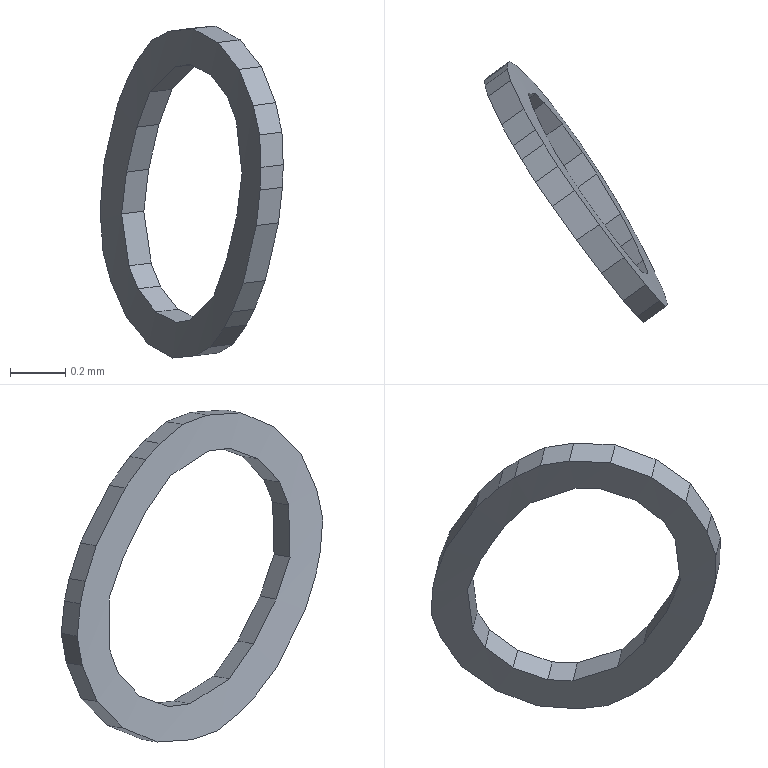Part | SolidWorks | features BaseBody 1 | 1 solid | 46 faces | box 0.6635 x 0.9504 x 1.207 mm | volume 0.04104 mm3 | plane 44 | cylinder 2 | commonest cylinder face diameters 16.8 x1 17 x1